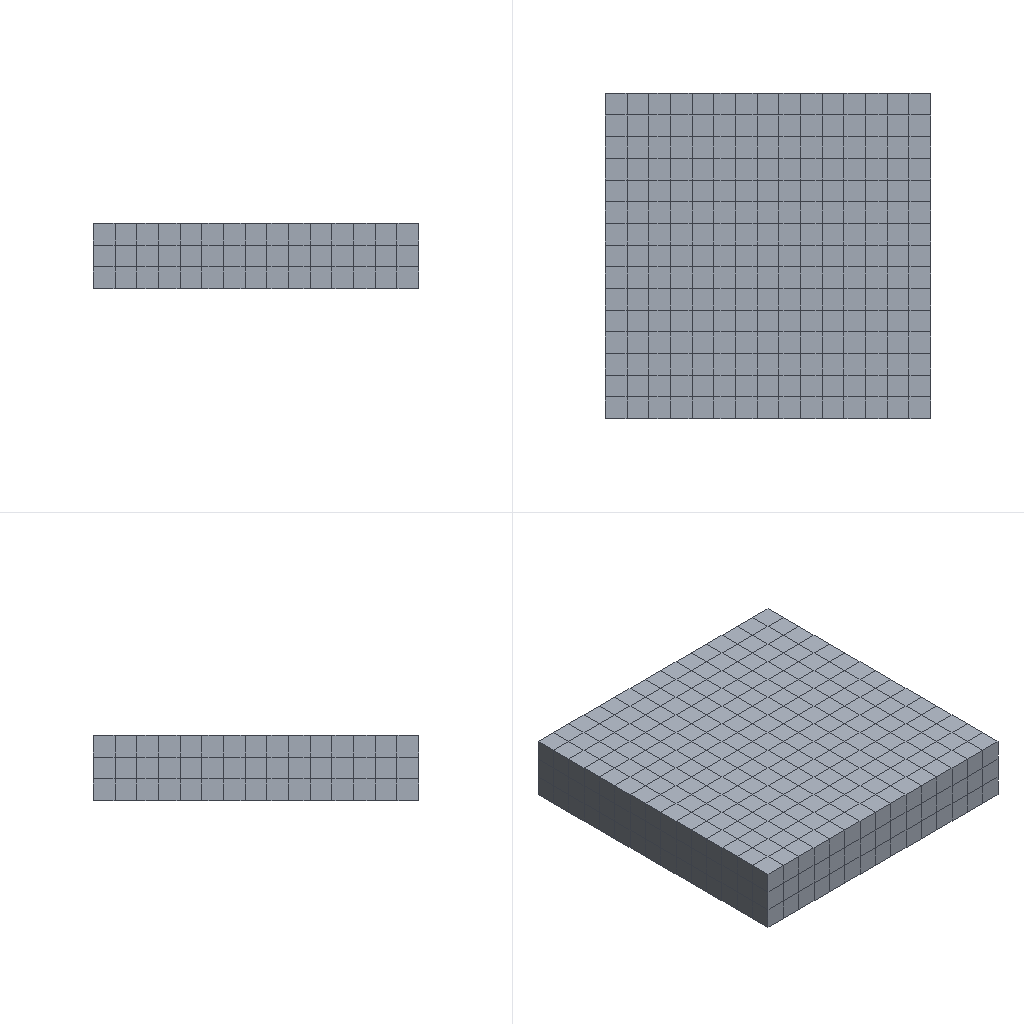Simulation study | ansys workbench
Set-up summary:
category,name,step,type,value,unit,region
solver,ansys_workbench
units,mm-N-s-tonne (MPa),,stated,"/units,MPA"
analysis,deck-1/LS1,,static
load_step,deck-1/LS1,deck-1/LS1,static,nsubst=1; time=1
analysis,deck-2/LS1,,static
load_step,deck-2/LS1,deck-2/LS1,static,nsubst=1; time=1
mesh,deck-1.dat,,nodes,16947
mesh,deck-1.dat,,elements,3710
element_type,SOLID186,,,3460,,deck-1.dat
element_type,SURF154,,,250,,deck-1.dat
mesh,deck-2.dat,,nodes,3712
mesh,deck-2.dat,,elements,765
element_type,SOLID186,,,675,,deck-2.dat
element_type,SURF154,,,90,,deck-2.dat
material,6061,,E,207000,tonne s^-2 mm^-1
material,6061,,nu,0.33
material,6061,,density,2.7e-09,tonne mm^-3
material,6061,,conductivity,60.5,tonne mm s^-3 C^-1
material,6061,,specific_heat,4.34e+08,mm^2 s^-2 C^-1
material,6061,,cte,2.34e-05,C^-1
material,6061,,permeability,10000
material,6061,,resistivity,0.00017,ohm mm
material,Structural Steel,,E,200000,tonne s^-2 mm^-1
material,Structural Steel,,nu,0.3
material,Structural Steel,,density,7.85e-09,tonne mm^-3
material,Structural Steel,,conductivity,60.5,tonne mm s^-3 C^-1
material,Structural Steel,,specific_heat,4.34e+08,mm^2 s^-2 C^-1
material,Structural Steel,,cte,1.2e-05,C^-1
material,Structural Steel,,permeability,10000
material,Structural Steel,,resistivity,0.00017,ohm mm
load,"Define Pressure Using Surface Effect Elements ""__""",deck-1/LS1,pressure,-100,,SURF154 #2
load,"Define Pressure Using Surface Effect Elements ""__ 2""",deck-1/LS1,pressure,-100,,SURF154 #3
load,"Define Pressure Using Surface Effect Elements ""__""",deck-2/LS1,pressure,-100,,SURF154 #2
load,"Define Pressure Using Surface Effect Elements ""__ 2""",deck-2/LS1,pressure,-100,,SURF154 #3
bc,Fixed Supports,deck-1/model,fixed,[dofs=ALL],,_FIXEDSU
bc,Fixed Supports,deck-2/model,fixed,[dofs=ALL],,_FIXEDSU
named_set,C_33,,node,453
named_set,_FIXEDSU,,node,419
named_set,_FIXEDSU,,node,172
Results summary:
result,analyses[0].index,,,1
result,analyses[0].system,,,SYS
result,analyses[0].deck,,,deck-1.dat
result,analyses[0].solve_status,,,completed
result,analyses[0].analysis_type,,,static
result,analyses[0].physics,,,mechanical
result,analyses[0].unit_system,,,"NMM: mm, ton, N, s, mV, mA, degC"
result,analyses[0].n_sets,,,1
result,analyses[0].load_steps[0].set,set=1,,1
result,analyses[0].load_steps[0].time_or_freq,set=1,,1
result,analyses[0].load_steps[0].max_displacement_magnitude,set=1,,0.08583
result,analyses[0].load_steps[0].max_von_mises_nodal,set=1,,1052.15
result,analyses[0].load_steps[0].reaction_force_sum_xyz[1],set=1,,-0.0001536
result,analyses[0].load_steps[0].reaction_force_sum_xyz[2],set=1,,-5.04614e-06
result,analyses[0].load_steps[0].reaction_force_sum_xyz[3],set=1,,-4.46219e-06
result,analyses[1].index,,,2
result,analyses[1].system,,,SYS-1
result,analyses[1].deck,,,deck-2.dat
result,analyses[1].solve_status,,,completed
result,analyses[1].analysis_type,,,static
result,analyses[1].physics,,,mechanical
result,analyses[1].unit_system,,,"NMM: mm, ton, N, s, mV, mA, degC"
result,analyses[1].n_sets,,,1
result,analyses[1].load_steps[0].set,set=1,,1
result,analyses[1].load_steps[0].time_or_freq,set=1,,1
result,analyses[1].load_steps[0].max_displacement_magnitude,set=1,,0.01468
result,analyses[1].load_steps[0].max_von_mises_nodal,set=1,,304.106
result,analyses[1].load_steps[0].reaction_force_sum_xyz[1],set=1,,7.8922e-05
result,analyses[1].load_steps[0].reaction_force_sum_xyz[2],set=1,,1.9188e-05
result,analyses[1].load_steps[0].reaction_force_sum_xyz[3],set=1,,2.00706e-05